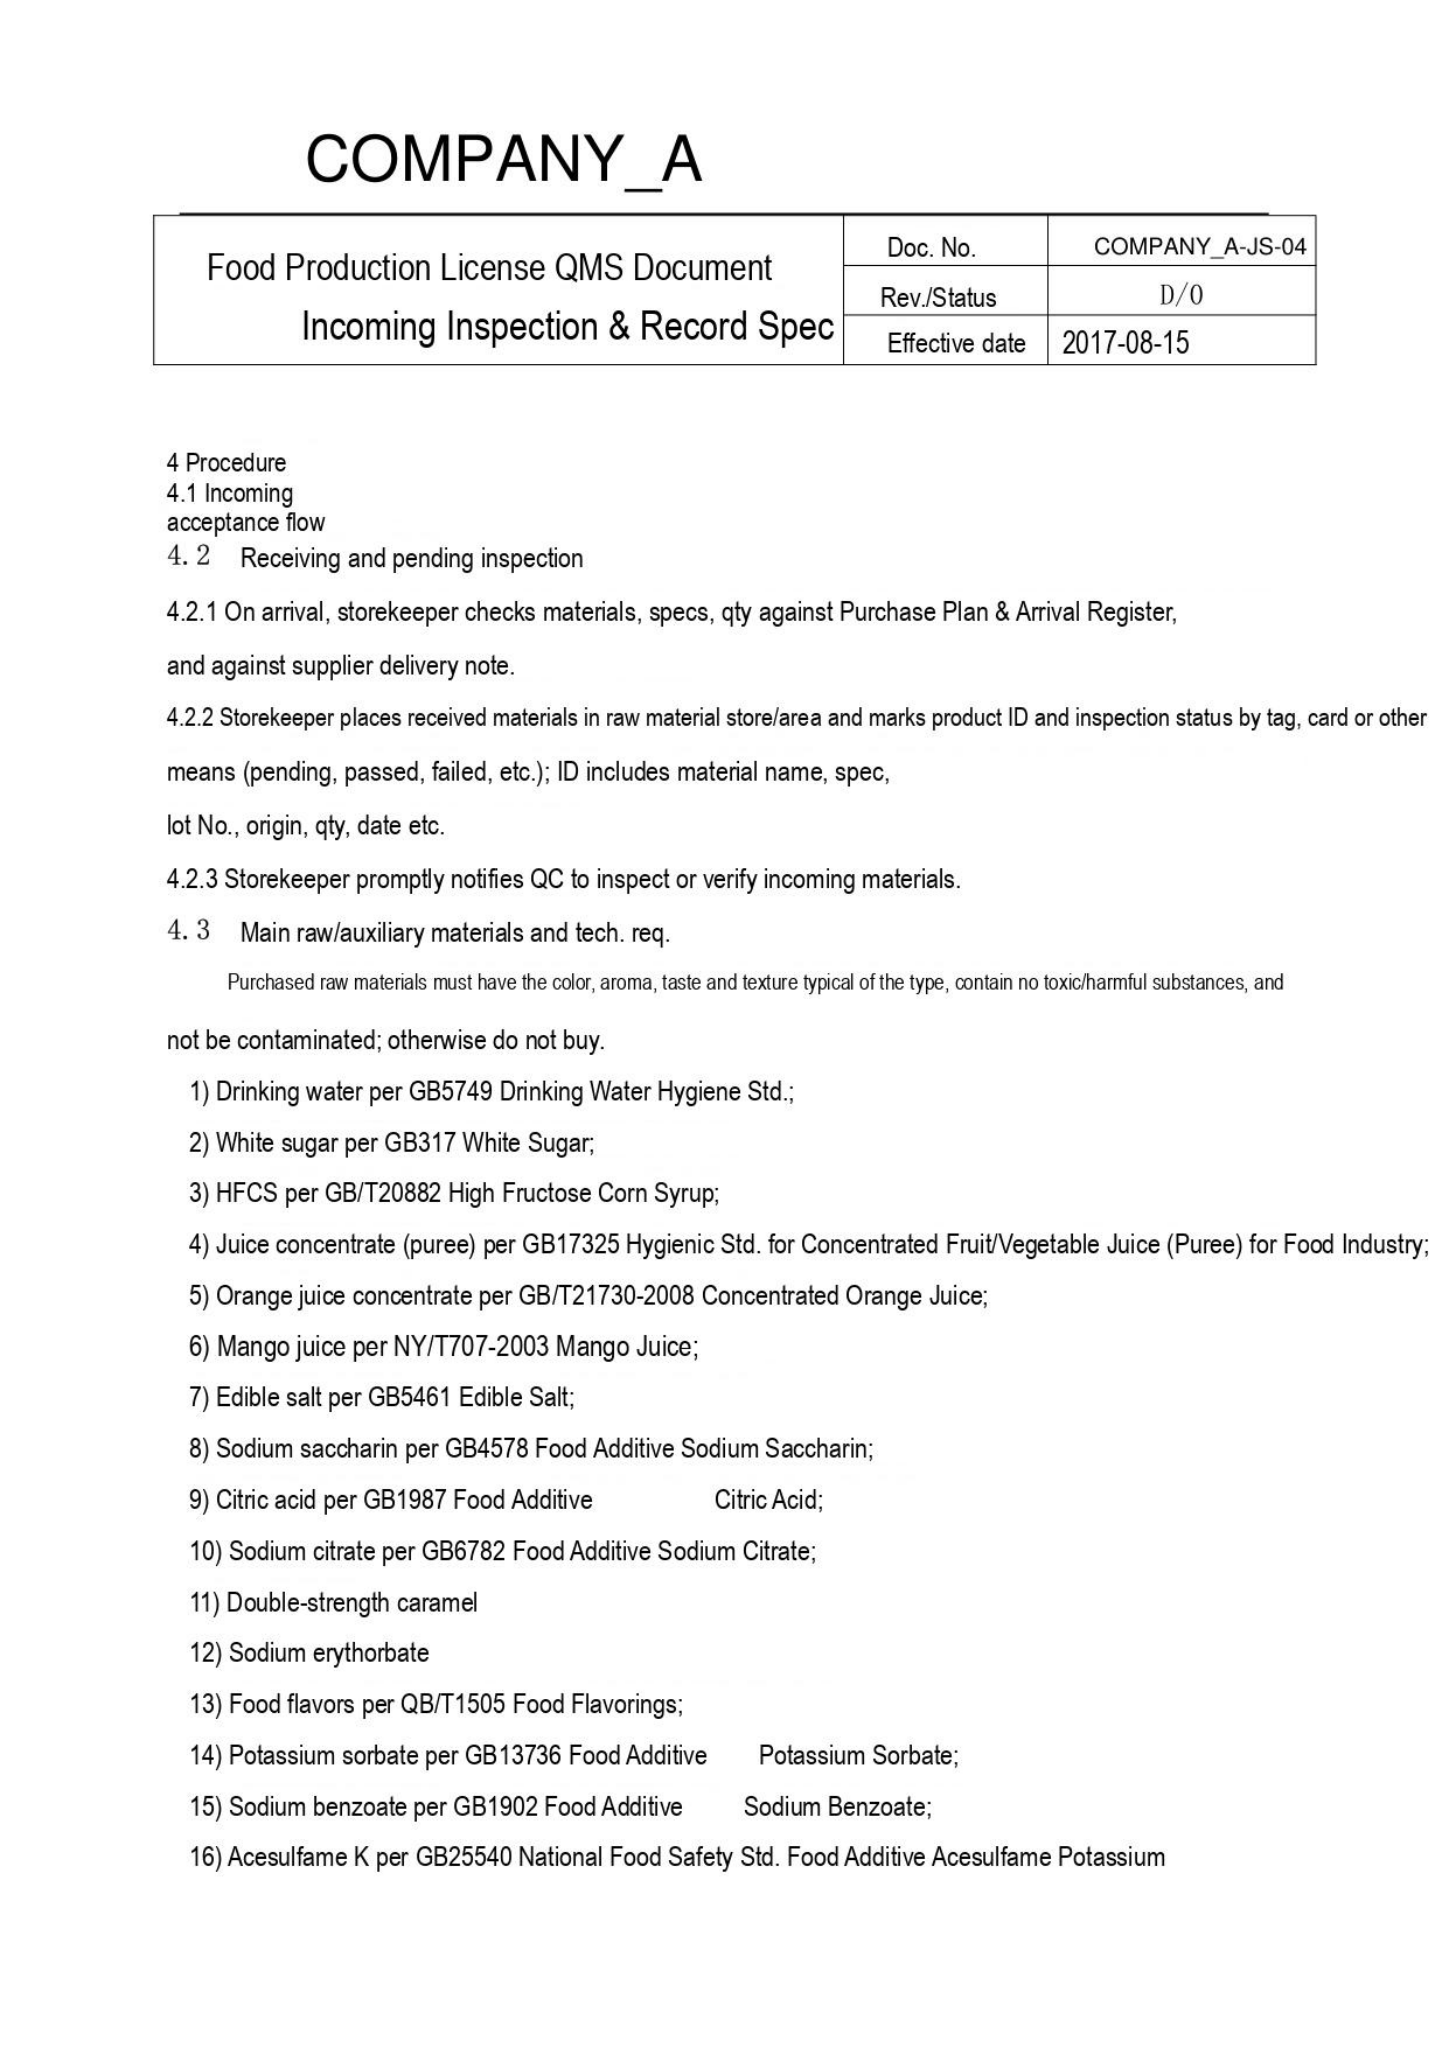COMPANY_A

| Food Production License QMS Document Incoming Inspection & Record Spec | Doc. No. | COMPANY_A-JS-04 |
|---|---|---|
| | Rev./Status | D/0 |
| | Effective date | 2017-08-15 |

4 Procedure
4.1 Incoming acceptance flow
4.2 Receiving and pending inspection

4.2.1 On arrival, storekeeper checks materials, specs, qty against Purchase Plan & Arrival Register, and against supplier delivery note.

4.2.2 Storekeeper places received materials in raw material store/area and marks product ID and inspection status by tag, card or other means (pending, passed, failed, etc.); ID includes material name, spec, lot No., origin, qty, date etc.

4.2.3 Storekeeper promptly notifies QC to inspect or verify incoming materials.

4.3 Main raw/auxiliary materials and tech. req.

Purchased raw materials must have the color, aroma, taste and texture typical of the type, contain no toxic/harmful substances, and not be contaminated; otherwise do not buy.

1) Drinking water per GB5749 Drinking Water Hygiene Std.;

2) White sugar per GB317 White Sugar;

3) HFCS per GB/T20882 High Fructose Corn Syrup;

4) Juice concentrate (puree) per GB17325 Hygienic Std. for Concentrated Fruit/Vegetable Juice (Puree) for Food Industry;

5) Orange juice concentrate per GB/T21730-2008 Concentrated Orange Juice;

6) Mango juice per NY/T707-2003 Mango Juice;

7) Edible salt per GB5461 Edible Salt;

8) Sodium saccharin per GB4578 Food Additive Sodium Saccharin;

9) Citric acid per GB1987 Food Additive Citric Acid;

10) Sodium citrate per GB6782 Food Additive Sodium Citrate;

11) Double-strength caramel

12) Sodium erythorbate

13) Food flavors per QB/T1505 Food Flavorings;

14) Potassium sorbate per GB13736 Food Additive Potassium Sorbate;

15) Sodium benzoate per GB1902 Food Additive Sodium Benzoate;

16) Acesulfame K per GB25540 National Food Safety Std. Food Additive Acesulfame Potassium
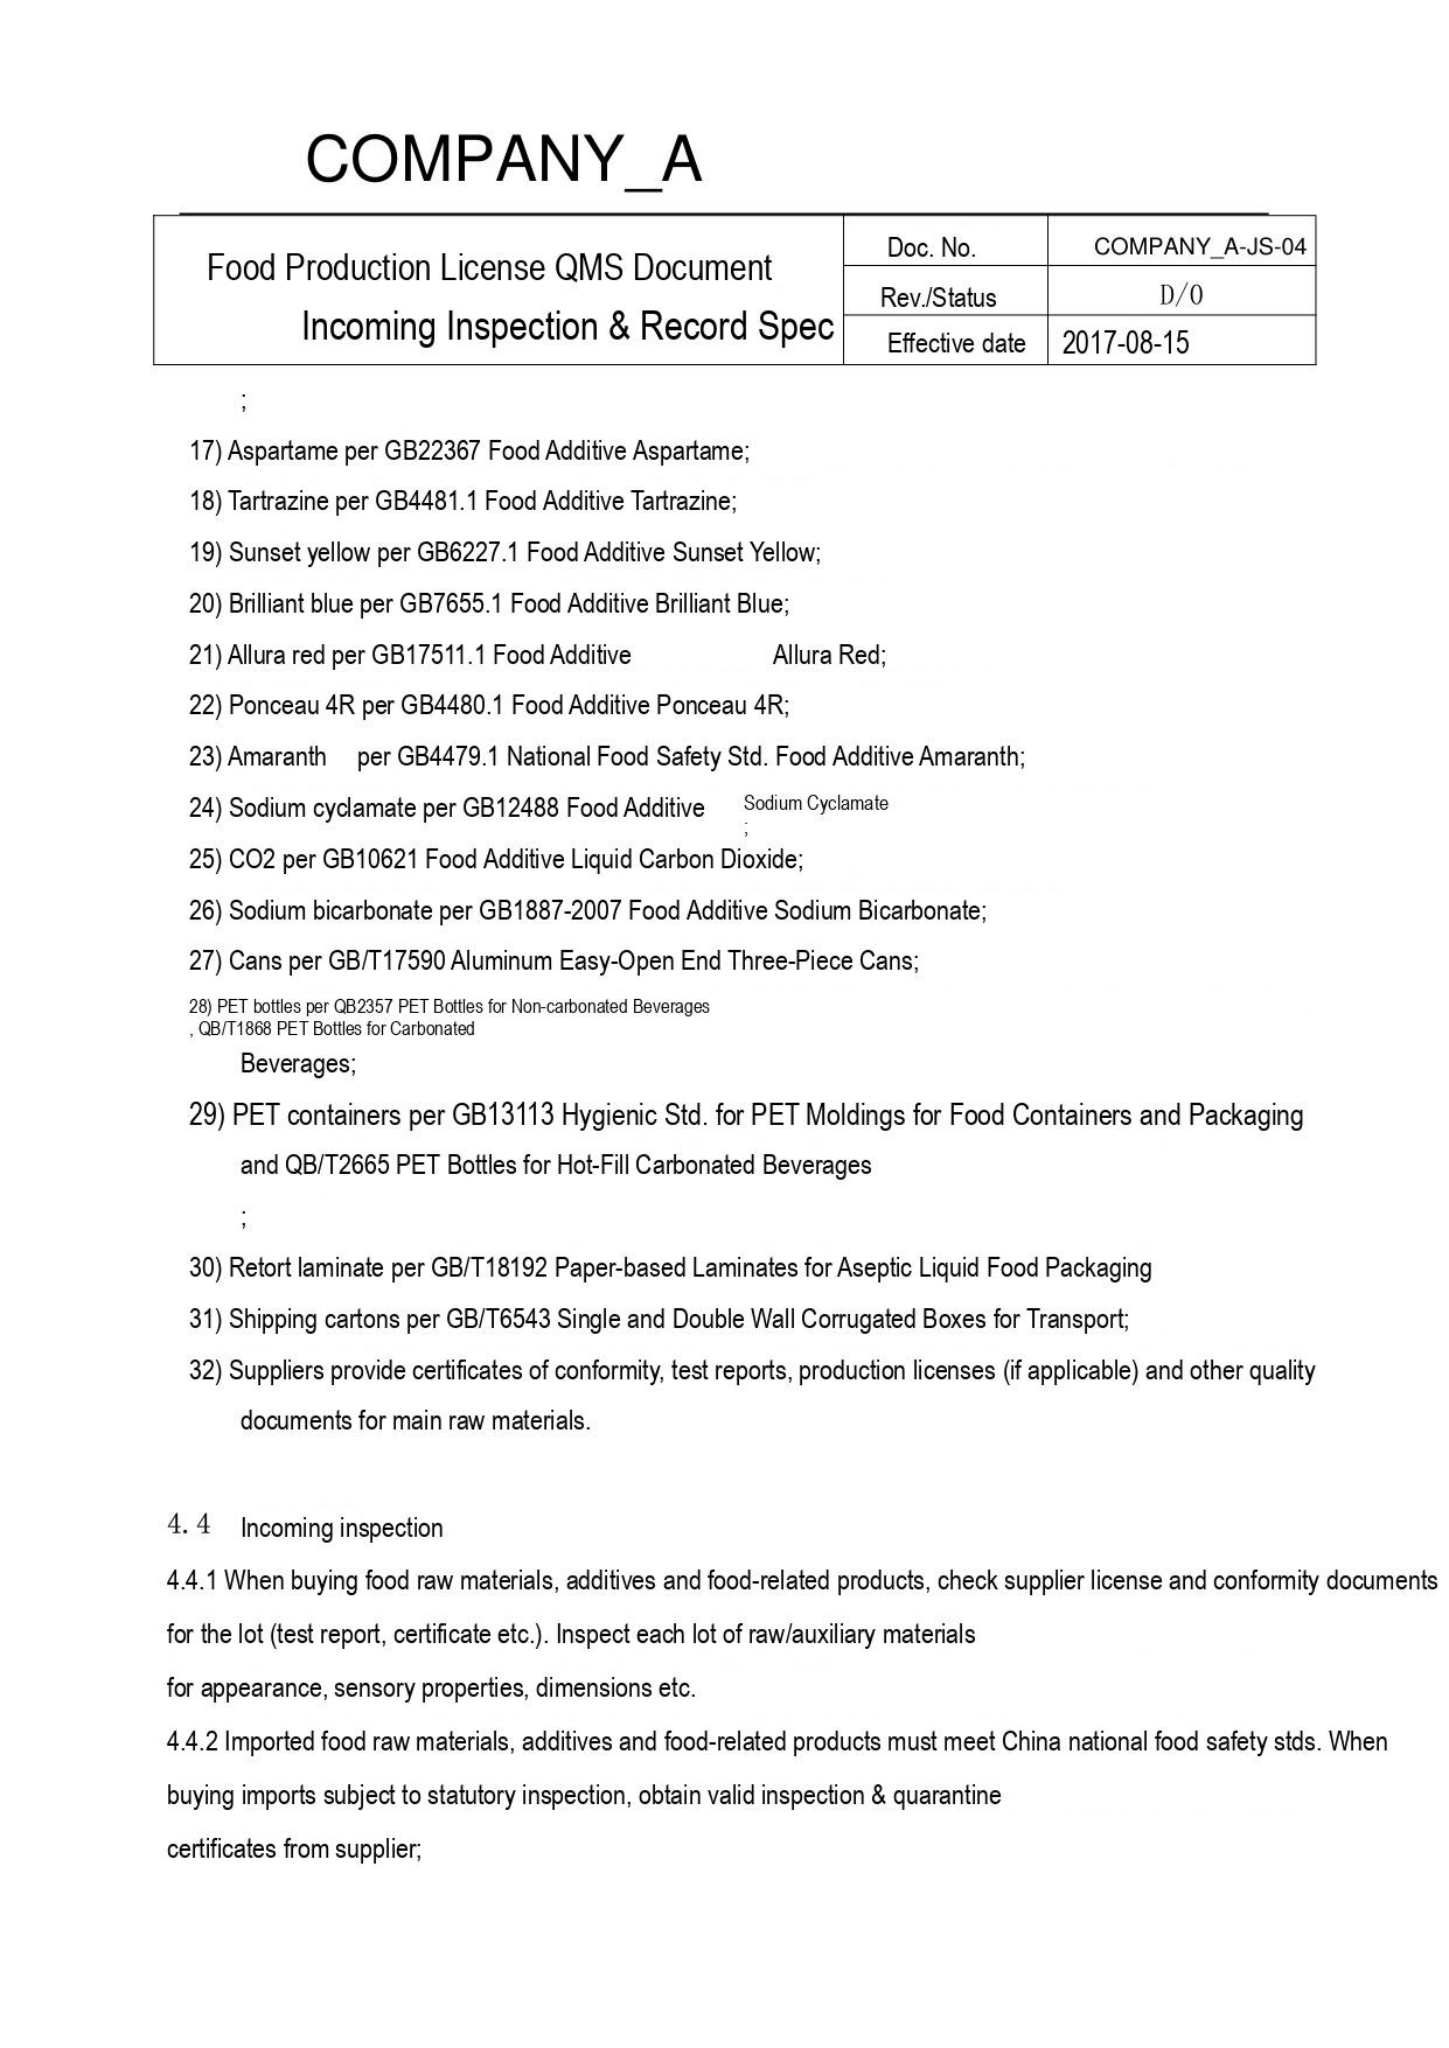COMPANY_A

| Food Production License QMS Document Incoming Inspection & Record Spec | Doc. No. | COMPANY_A-JS-04 |
|---|---|---|
| | Rev./Status | D/0 |
| | Effective date | 2017-08-15 |

;

17) Aspartame per GB22367 Food Additive Aspartame;

18) Tartrazine per GB4481.1 Food Additive Tartrazine;

19) Sunset yellow per GB6227.1 Food Additive Sunset Yellow;

20) Brilliant blue per GB7655.1 Food Additive Brilliant Blue;

21) Allura red per GB17511.1 Food Additive Allura Red;

22) Ponceau 4R per GB4480.1 Food Additive Ponceau 4R;

23) Amaranth per GB4479.1 National Food Safety Std. Food Additive Amaranth;

24) Sodium cyclamate per GB12488 Food Additive Sodium Cyclamate ;

25) CO2 per GB10621 Food Additive Liquid Carbon Dioxide;

26) Sodium bicarbonate per GB1887-2007 Food Additive Sodium Bicarbonate;

27) Cans per GB/T17590 Aluminum Easy-Open End Three-Piece Cans;

28) PET bottles per QB2357 PET Bottles for Non-carbonated Beverages , QB/T1868 PET Bottles for Carbonated Beverages;

29) PET containers per GB13113 Hygienic Std. for PET Moldings for Food Containers and Packaging and QB/T2665 PET Bottles for Hot-Fill Carbonated Beverages ;

30) Retort laminate per GB/T18192 Paper-based Laminates for Aseptic Liquid Food Packaging

31) Shipping cartons per GB/T6543 Single and Double Wall Corrugated Boxes for Transport;

32) Suppliers provide certificates of conformity, test reports, production licenses (if applicable) and other quality documents for main raw materials.

4.4 Incoming inspection

4.4.1 When buying food raw materials, additives and food-related products, check supplier license and conformity documents for the lot (test report, certificate etc.). Inspect each lot of raw/auxiliary materials for appearance, sensory properties, dimensions etc.

4.4.2 Imported food raw materials, additives and food-related products must meet China national food safety stds. When buying imports subject to statutory inspection, obtain valid inspection & quarantine certificates from supplier;
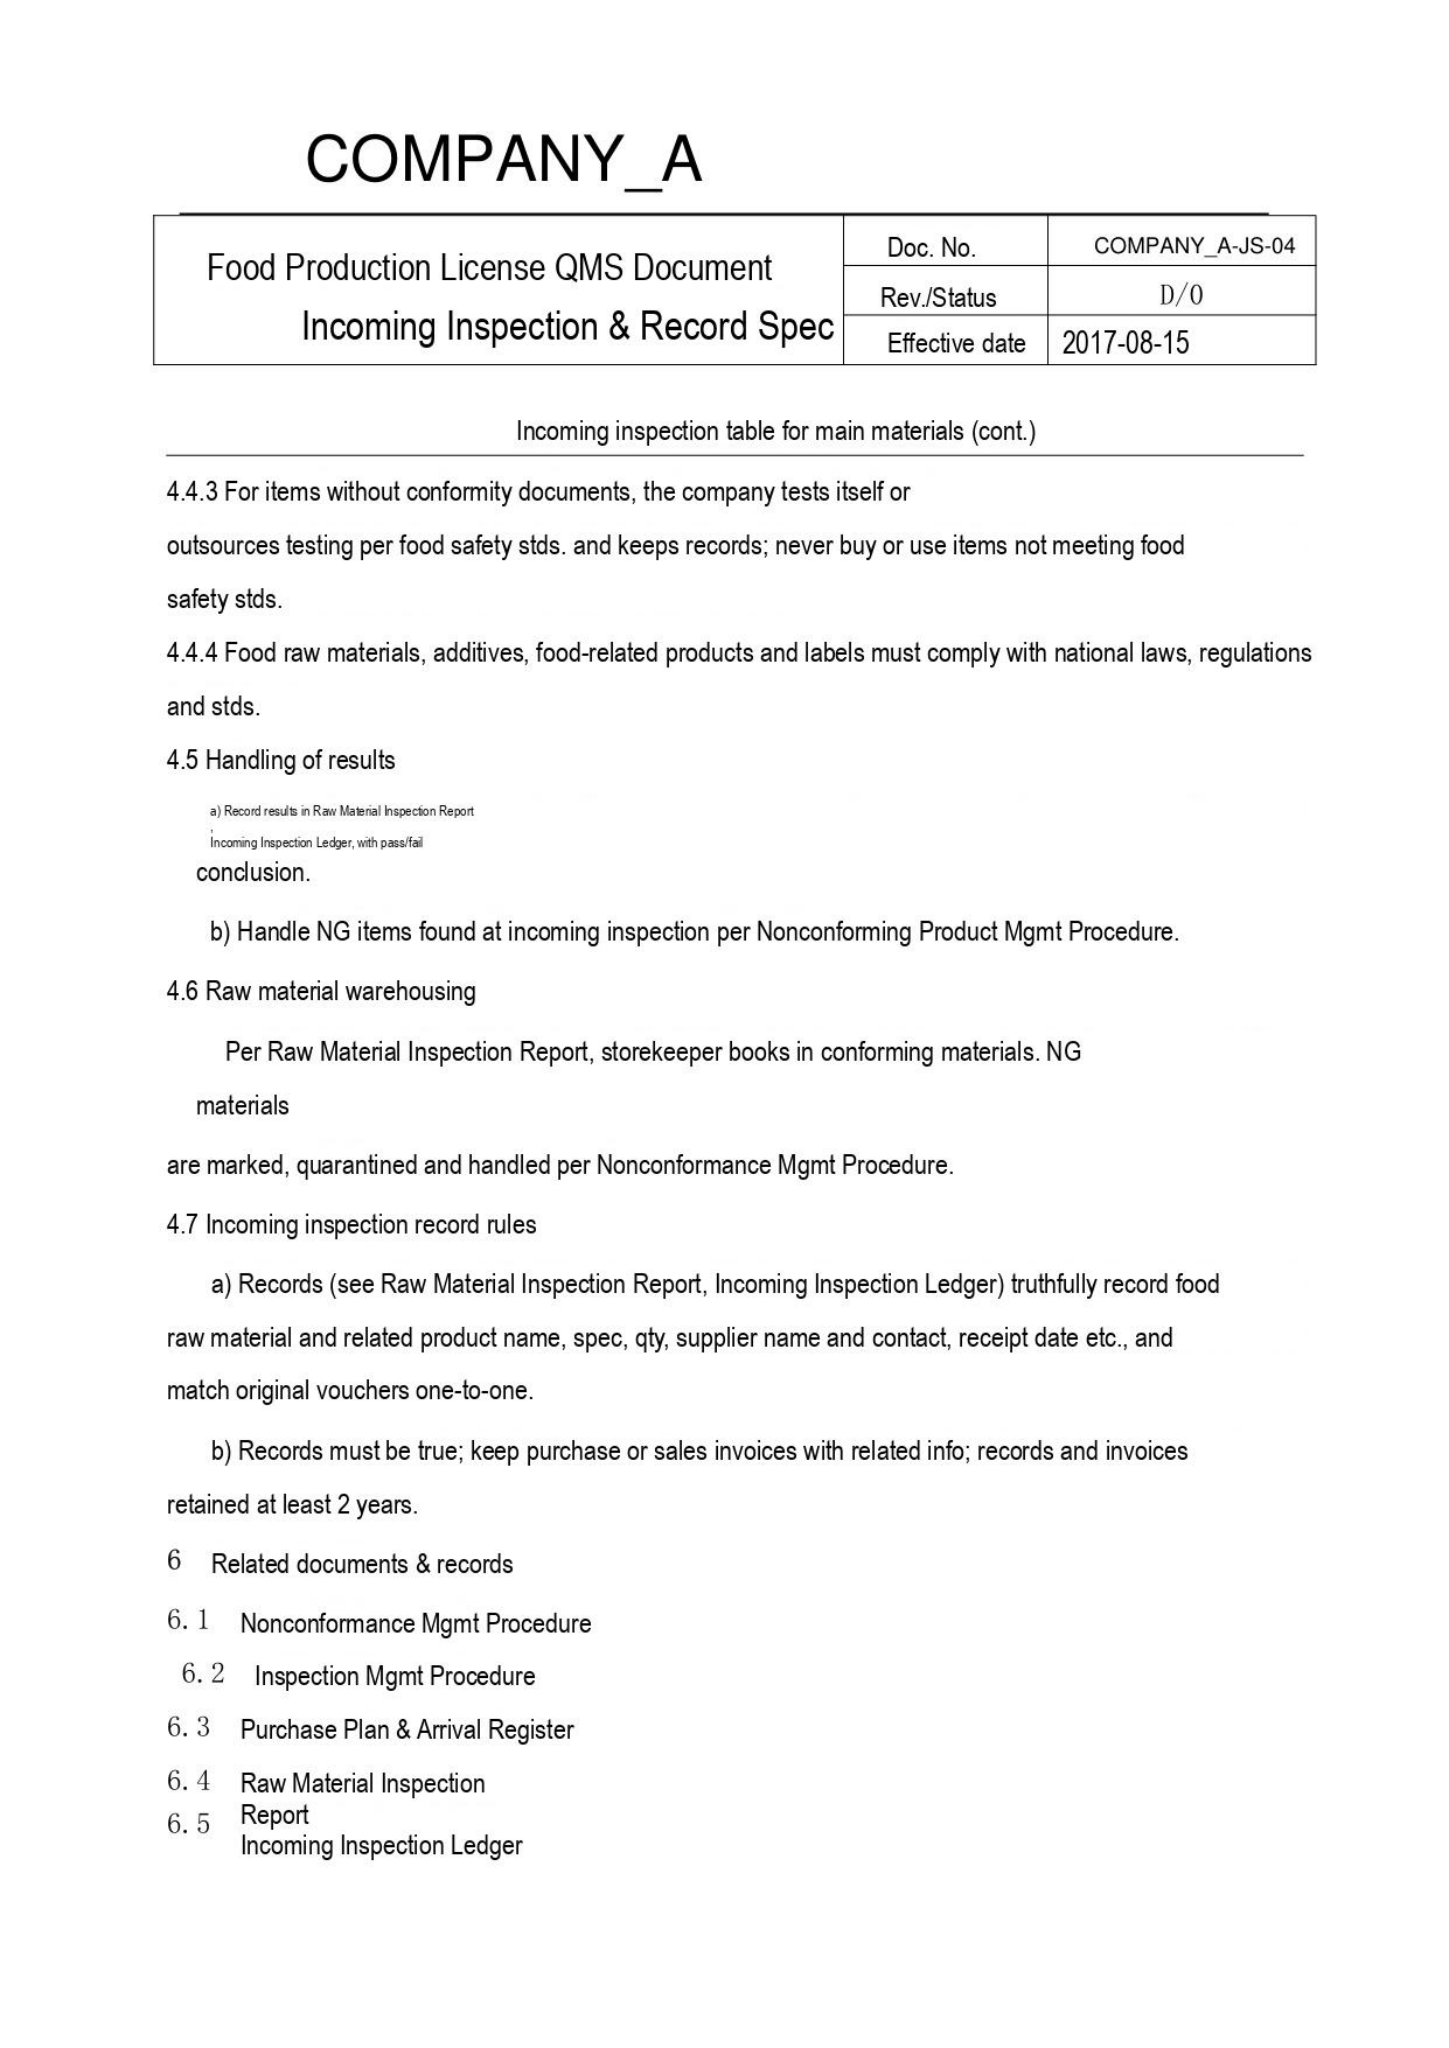COMPANY_A

| Food Production License QMS Document<br>Incoming Inspection & Record Spec | Doc. No. | COMPANY_A-JS-04 |
|---|---|---|
| | Rev./Status | D/0 |
| | Effective date | 2017-08-15 |

Incoming inspection table for main materials (cont.)

4.4.3 For items without conformity documents, the company tests itself or outsources testing per food safety stds. and keeps records; never buy or use items not meeting food safety stds.

4.4.4 Food raw materials, additives, food-related products and labels must comply with national laws, regulations and stds.

4.5 Handling of results

a) Record results in Raw Material Inspection Report Incoming Inspection Ledger, with pass/fail conclusion.

b) Handle NG items found at incoming inspection per Nonconforming Product Mgmt Procedure.

4.6 Raw material warehousing

Per Raw Material Inspection Report, storekeeper books in conforming materials. NG materials are marked, quarantined and handled per Nonconformance Mgmt Procedure.

4.7 Incoming inspection record rules

a) Records (see Raw Material Inspection Report, Incoming Inspection Ledger) truthfully record food raw material and related product name, spec, qty, supplier name and contact, receipt date etc., and match original vouchers one-to-one.

b) Records must be true; keep purchase or sales invoices with related info; records and invoices retained at least 2 years.

6 Related documents & records

6.1 Nonconformance Mgmt Procedure

6.2 Inspection Mgmt Procedure

6.3 Purchase Plan & Arrival Register

6.4 Raw Material Inspection Report

6.5 Incoming Inspection Ledger